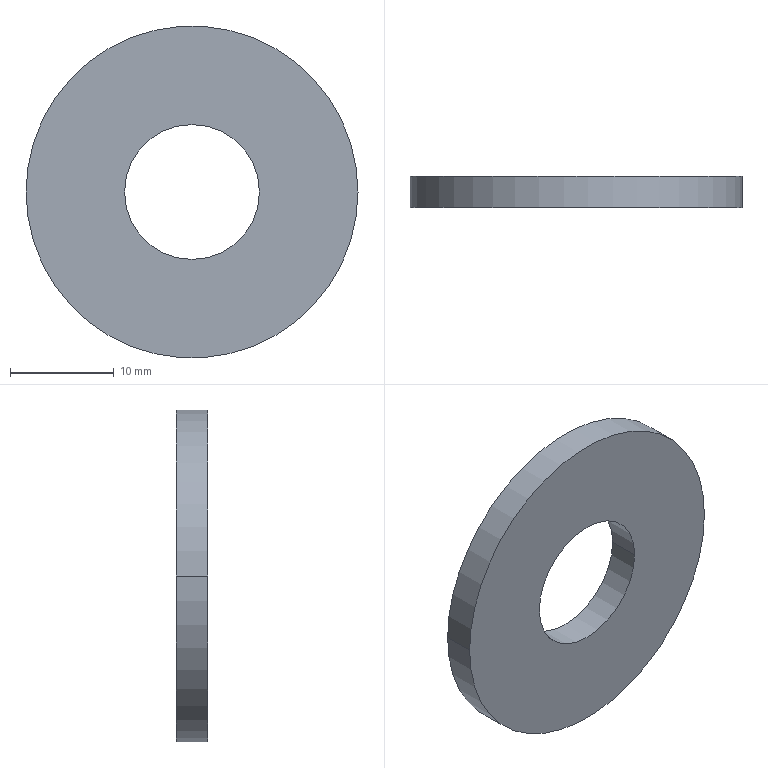Part | STEP file | LIB_26379326_WASHER_M12 | 1 solid | 6 faces | box 32 x 3 x 32 mm | volume 2015 mm3 | cylinder 4 | plane 2 | commonest cylinder face diameters 13 x2 32 x2
STEP:
#1=CARTESIAN_POINT('',(0.,0.,0.));
#2=DIRECTION('',(0.,0.,1.));
#3=DIRECTION('',(1.,0.,0.));
#4=AXIS2_PLACEMENT_3D('',#1,#2,#3);
#5=CARTESIAN_POINT('',(16.,0.,0.));
#6=VERTEX_POINT('',#5);
#7=CARTESIAN_POINT('',(-16.,0.,0.));
#8=VERTEX_POINT('',#7);
#9=CARTESIAN_POINT('',(0.,0.,0.));
#10=DIRECTION('',(0.,1.,0.));
#11=DIRECTION('',(1.,0.,0.));
#12=AXIS2_PLACEMENT_3D('',#9,#10,#11);
#13=CIRCLE('',#12,16.);
#14=CARTESIAN_POINT('',(0.,0.,0.));
#15=DIRECTION('',(0.,1.,0.));
#16=DIRECTION('',(1.,0.,0.));
#17=AXIS2_PLACEMENT_3D('',#14,#15,#16);
#18=PLANE('',#17);
#19=CARTESIAN_POINT('',(0.,0.));
#20=DIRECTION('',(1.,0.));
#21=AXIS2_PLACEMENT_2D('',#19,#20);
#22=CIRCLE('',#21,16.);
#23=(GEOMETRIC_REPRESENTATION_CONTEXT(2)PARAMETRIC_REPRESENTATION_CONTEXT()REPRESENTATION_CONTEXT('',''));
#24=DEFINITIONAL_REPRESENTATION('',(#22),#23);
#25=PCURVE('',#18,#24);
#26=CARTESIAN_POINT('',(0.,0.,0.));
#27=DIRECTION('',(0.,1.,0.));
#28=DIRECTION('',(1.,0.,0.));
#29=AXIS2_PLACEMENT_3D('',#26,#27,#28);
#30=CYLINDRICAL_SURFACE('',#29,16.);
#31=CARTESIAN_POINT('',(0.,0.));
#32=DIRECTION('',(1.,0.));
#33=VECTOR('',#32,1.);
#34=LINE('',#31,#33);
#35=(GEOMETRIC_REPRESENTATION_CONTEXT(2)PARAMETRIC_REPRESENTATION_CONTEXT()REPRESENTATION_CONTEXT('',''));
#36=DEFINITIONAL_REPRESENTATION('',(#34),#35);
#37=PCURVE('',#30,#36);
#38=SURFACE_CURVE('',#13,(#25,#37),.PCURVE_S1.);
#39=EDGE_CURVE('',#6,#8,#38,.T.);
#40=ORIENTED_EDGE('',*,*,#39,.T.);
#41=CARTESIAN_POINT('',(0.,0.,0.));
#42=DIRECTION('',(0.,1.,0.));
#43=DIRECTION('',(-1.,0.,0.));
#44=AXIS2_PLACEMENT_3D('',#41,#42,#43);
#45=CIRCLE('',#44,16.);
#46=CARTESIAN_POINT('',(0.,0.));
#47=DIRECTION('',(-1.,0.));
#48=AXIS2_PLACEMENT_2D('',#46,#47);
#49=CIRCLE('',#48,16.);
#50=(GEOMETRIC_REPRESENTATION_CONTEXT(2)PARAMETRIC_REPRESENTATION_CONTEXT()REPRESENTATION_CONTEXT('',''));
#51=DEFINITIONAL_REPRESENTATION('',(#49),#50);
#52=PCURVE('',#18,#51);
#53=CARTESIAN_POINT('',(0.,0.,0.));
#54=DIRECTION('',(0.,1.,0.));
#55=DIRECTION('',(1.,0.,0.));
#56=AXIS2_PLACEMENT_3D('',#53,#54,#55);
#57=CYLINDRICAL_SURFACE('',#56,16.);
#58=CARTESIAN_POINT('',(3.142,0.));
#59=DIRECTION('',(1.,0.));
#60=VECTOR('',#59,1.);
#61=LINE('',#58,#60);
#62=(GEOMETRIC_REPRESENTATION_CONTEXT(2)PARAMETRIC_REPRESENTATION_CONTEXT()REPRESENTATION_CONTEXT('',''));
#63=DEFINITIONAL_REPRESENTATION('',(#61),#62);
#64=PCURVE('',#57,#63);
#65=SURFACE_CURVE('',#45,(#52,#64),.PCURVE_S1.);
#66=EDGE_CURVE('',#8,#6,#65,.T.);
#67=ORIENTED_EDGE('',*,*,#66,.T.);
#68=EDGE_LOOP('',(#40,#67));
#69=FACE_BOUND('',#68,.F.);
#70=CARTESIAN_POINT('',(6.5,0.,0.));
#71=VERTEX_POINT('',#70);
#72=CARTESIAN_POINT('',(-6.5,0.,0.));
#73=VERTEX_POINT('',#72);
#74=CARTESIAN_POINT('',(0.,0.,0.));
#75=DIRECTION('',(0.,-1.,0.));
#76=DIRECTION('',(1.,0.,0.));
#77=AXIS2_PLACEMENT_3D('',#74,#75,#76);
#78=CIRCLE('',#77,6.5);
#79=CARTESIAN_POINT('',(6.5,0.));
#80=CARTESIAN_POINT('',(6.5,-11.258));
#81=CARTESIAN_POINT('',(-3.25,-5.629));
#82=CARTESIAN_POINT('',(-13.,0.));
#83=CARTESIAN_POINT('',(-3.25,5.629));
#84=CARTESIAN_POINT('',(6.5,11.258));
#85=CARTESIAN_POINT('',(6.5,0.));
#86=(BOUNDED_CURVE()B_SPLINE_CURVE(2,(#79,#80,#81,#82,#83,#84,#85),.UNSPECIFIED.,.T.,.F.)B_SPLINE_CURVE_WITH_KNOTS((1,2,2,2,2,1),(-2.094,0.,2.094,4.189,6.283,8.378),.UNSPECIFIED.)CURVE()GEOMETRIC_REPRESENTATION_ITEM()RATIONAL_B_SPLINE_CURVE((1.,0.5,1.,0.5,1.,0.5,1.))REPRESENTATION_ITEM(''));
#87=(GEOMETRIC_REPRESENTATION_CONTEXT(2)PARAMETRIC_REPRESENTATION_CONTEXT()REPRESENTATION_CONTEXT('',''));
#88=DEFINITIONAL_REPRESENTATION('',(#86),#87);
#89=PCURVE('',#18,#88);
#90=CARTESIAN_POINT('',(0.,0.,0.));
#91=DIRECTION('',(0.,1.,0.));
#92=DIRECTION('',(1.,0.,0.));
#93=AXIS2_PLACEMENT_3D('',#90,#91,#92);
#94=CYLINDRICAL_SURFACE('',#93,6.5);
#95=CARTESIAN_POINT('',(6.283,0.));
#96=DIRECTION('',(-1.,0.));
#97=VECTOR('',#96,1.);
#98=LINE('',#95,#97);
#99=(GEOMETRIC_REPRESENTATION_CONTEXT(2)PARAMETRIC_REPRESENTATION_CONTEXT()REPRESENTATION_CONTEXT('',''));
#100=DEFINITIONAL_REPRESENTATION('',(#98),#99);
#101=PCURVE('',#94,#100);
#102=SURFACE_CURVE('',#78,(#89,#101),.PCURVE_S1.);
#103=EDGE_CURVE('',#71,#73,#102,.T.);
#104=ORIENTED_EDGE('',*,*,#103,.T.);
#105=CARTESIAN_POINT('',(0.,0.,0.));
#106=DIRECTION('',(0.,-1.,0.));
#107=DIRECTION('',(-1.,0.,0.));
#108=AXIS2_PLACEMENT_3D('',#105,#106,#107);
#109=CIRCLE('',#108,6.5);
#110=CARTESIAN_POINT('',(-6.5,0.));
#111=CARTESIAN_POINT('',(-6.5,11.258));
#112=CARTESIAN_POINT('',(3.25,5.629));
#113=CARTESIAN_POINT('',(13.,0.));
#114=CARTESIAN_POINT('',(3.25,-5.629));
#115=CARTESIAN_POINT('',(-6.5,-11.258));
#116=CARTESIAN_POINT('',(-6.5,0.));
#117=(BOUNDED_CURVE()B_SPLINE_CURVE(2,(#110,#111,#112,#113,#114,#115,#116),.UNSPECIFIED.,.T.,.F.)B_SPLINE_CURVE_WITH_KNOTS((1,2,2,2,2,1),(-2.094,0.,2.094,4.189,6.283,8.378),.UNSPECIFIED.)CURVE()GEOMETRIC_REPRESENTATION_ITEM()RATIONAL_B_SPLINE_CURVE((1.,0.5,1.,0.5,1.,0.5,1.))REPRESENTATION_ITEM(''));
#118=(GEOMETRIC_REPRESENTATION_CONTEXT(2)PARAMETRIC_REPRESENTATION_CONTEXT()REPRESENTATION_CONTEXT('',''));
#119=DEFINITIONAL_REPRESENTATION('',(#117),#118);
#120=PCURVE('',#18,#119);
#121=CARTESIAN_POINT('',(0.,0.,0.));
#122=DIRECTION('',(0.,1.,0.));
#123=DIRECTION('',(1.,0.,0.));
#124=AXIS2_PLACEMENT_3D('',#121,#122,#123);
#125=CYLINDRICAL_SURFACE('',#124,6.5);
#126=CARTESIAN_POINT('',(3.142,0.));
#127=DIRECTION('',(-1.,0.));
#128=VECTOR('',#127,1.);
#129=LINE('',#126,#128);
#130=(GEOMETRIC_REPRESENTATION_CONTEXT(2)PARAMETRIC_REPRESENTATION_CONTEXT()REPRESENTATION_CONTEXT('',''));
#131=DEFINITIONAL_REPRESENTATION('',(#129),#130);
#132=PCURVE('',#125,#131);
#133=SURFACE_CURVE('',#109,(#120,#132),.PCURVE_S1.);
#134=EDGE_CURVE('',#73,#71,#133,.T.);
#135=ORIENTED_EDGE('',*,*,#134,.T.);
#136=EDGE_LOOP('',(#104,#135));
#137=FACE_BOUND('',#136,.F.);
#138=ADVANCED_FACE('',(#69,#137),#18,.F.);
#139=CARTESIAN_POINT('',(-16.,3.,0.));
#140=VERTEX_POINT('',#139);
#141=CARTESIAN_POINT('',(-16.,0.,0.));
#142=DIRECTION('',(0.,1.,0.));
#143=VECTOR('',#142,1.);
#144=LINE('',#141,#143);
#145=CARTESIAN_POINT('',(3.142,0.));
#146=DIRECTION('',(0.,1.));
#147=VECTOR('',#146,1.);
#148=LINE('',#145,#147);
#149=(GEOMETRIC_REPRESENTATION_CONTEXT(2)PARAMETRIC_REPRESENTATION_CONTEXT()REPRESENTATION_CONTEXT('',''));
#150=DEFINITIONAL_REPRESENTATION('',(#148),#149);
#151=PCURVE('',#30,#150);
#152=CARTESIAN_POINT('',(3.142,0.));
#153=DIRECTION('',(0.,1.));
#154=VECTOR('',#153,1.);
#155=LINE('',#152,#154);
#156=(GEOMETRIC_REPRESENTATION_CONTEXT(2)PARAMETRIC_REPRESENTATION_CONTEXT()REPRESENTATION_CONTEXT('',''));
#157=DEFINITIONAL_REPRESENTATION('',(#155),#156);
#158=PCURVE('',#57,#157);
#159=SURFACE_CURVE('',#144,(#151,#158),.PCURVE_S1.);
#160=EDGE_CURVE('',#8,#140,#159,.T.);
#161=ORIENTED_EDGE('',*,*,#160,.T.);
#162=CARTESIAN_POINT('',(16.,3.,0.));
#163=VERTEX_POINT('',#162);
#164=CARTESIAN_POINT('',(0.,3.,0.));
#165=DIRECTION('',(0.,1.,0.));
#166=DIRECTION('',(1.,0.,0.));
#167=AXIS2_PLACEMENT_3D('',#164,#165,#166);
#168=CIRCLE('',#167,16.);
#169=CARTESIAN_POINT('',(0.,3.));
#170=DIRECTION('',(1.,0.));
#171=VECTOR('',#170,1.);
#172=LINE('',#169,#171);
#173=(GEOMETRIC_REPRESENTATION_CONTEXT(2)PARAMETRIC_REPRESENTATION_CONTEXT()REPRESENTATION_CONTEXT('',''));
#174=DEFINITIONAL_REPRESENTATION('',(#172),#173);
#175=PCURVE('',#30,#174);
#176=CARTESIAN_POINT('',(0.,3.,0.));
#177=DIRECTION('',(0.,1.,0.));
#178=DIRECTION('',(1.,0.,0.));
#179=AXIS2_PLACEMENT_3D('',#176,#177,#178);
#180=PLANE('',#179);
#181=CARTESIAN_POINT('',(0.,0.));
#182=DIRECTION('',(1.,0.));
#183=AXIS2_PLACEMENT_2D('',#181,#182);
#184=CIRCLE('',#183,16.);
#185=(GEOMETRIC_REPRESENTATION_CONTEXT(2)PARAMETRIC_REPRESENTATION_CONTEXT()REPRESENTATION_CONTEXT('',''));
#186=DEFINITIONAL_REPRESENTATION('',(#184),#185);
#187=PCURVE('',#180,#186);
#188=SURFACE_CURVE('',#168,(#175,#187),.PCURVE_S1.);
#189=EDGE_CURVE('',#163,#140,#188,.T.);
#190=ORIENTED_EDGE('',*,*,#189,.F.);
#191=CARTESIAN_POINT('',(16.,0.,0.));
#192=DIRECTION('',(0.,1.,0.));
#193=VECTOR('',#192,1.);
#194=LINE('',#191,#193);
#195=CARTESIAN_POINT('',(0.,0.));
#196=DIRECTION('',(0.,1.));
#197=VECTOR('',#196,1.);
#198=LINE('',#195,#197);
#199=(GEOMETRIC_REPRESENTATION_CONTEXT(2)PARAMETRIC_REPRESENTATION_CONTEXT()REPRESENTATION_CONTEXT('',''));
#200=DEFINITIONAL_REPRESENTATION('',(#198),#199);
#201=PCURVE('',#30,#200);
#202=CARTESIAN_POINT('',(6.283,0.));
#203=DIRECTION('',(0.,1.));
#204=VECTOR('',#203,1.);
#205=LINE('',#202,#204);
#206=(GEOMETRIC_REPRESENTATION_CONTEXT(2)PARAMETRIC_REPRESENTATION_CONTEXT()REPRESENTATION_CONTEXT('',''));
#207=DEFINITIONAL_REPRESENTATION('',(#205),#206);
#208=PCURVE('',#57,#207);
#209=SURFACE_CURVE('',#194,(#201,#208),.PCURVE_S1.);
#210=EDGE_CURVE('',#6,#163,#209,.T.);
#211=ORIENTED_EDGE('',*,*,#210,.F.);
#212=ORIENTED_EDGE('',*,*,#39,.T.);
#213=EDGE_LOOP('',(#161,#190,#211,#212));
#214=FACE_BOUND('',#213,.T.);
#215=ADVANCED_FACE('',(#214),#30,.T.);
#216=ORIENTED_EDGE('',*,*,#210,.T.);
#217=CARTESIAN_POINT('',(0.,3.,0.));
#218=DIRECTION('',(0.,1.,0.));
#219=DIRECTION('',(-1.,0.,0.));
#220=AXIS2_PLACEMENT_3D('',#217,#218,#219);
#221=CIRCLE('',#220,16.);
#222=CARTESIAN_POINT('',(3.142,3.));
#223=DIRECTION('',(1.,0.));
#224=VECTOR('',#223,1.);
#225=LINE('',#222,#224);
#226=(GEOMETRIC_REPRESENTATION_CONTEXT(2)PARAMETRIC_REPRESENTATION_CONTEXT()REPRESENTATION_CONTEXT('',''));
#227=DEFINITIONAL_REPRESENTATION('',(#225),#226);
#228=PCURVE('',#57,#227);
#229=CARTESIAN_POINT('',(0.,0.));
#230=DIRECTION('',(-1.,0.));
#231=AXIS2_PLACEMENT_2D('',#229,#230);
#232=CIRCLE('',#231,16.);
#233=(GEOMETRIC_REPRESENTATION_CONTEXT(2)PARAMETRIC_REPRESENTATION_CONTEXT()REPRESENTATION_CONTEXT('',''));
#234=DEFINITIONAL_REPRESENTATION('',(#232),#233);
#235=PCURVE('',#180,#234);
#236=SURFACE_CURVE('',#221,(#228,#235),.PCURVE_S1.);
#237=EDGE_CURVE('',#140,#163,#236,.T.);
#238=ORIENTED_EDGE('',*,*,#237,.F.);
#239=ORIENTED_EDGE('',*,*,#160,.F.);
#240=ORIENTED_EDGE('',*,*,#66,.T.);
#241=EDGE_LOOP('',(#216,#238,#239,#240));
#242=FACE_BOUND('',#241,.T.);
#243=ADVANCED_FACE('',(#242),#57,.T.);
#244=ORIENTED_EDGE('',*,*,#189,.F.);
#245=ORIENTED_EDGE('',*,*,#237,.F.);
#246=EDGE_LOOP('',(#244,#245));
#247=FACE_BOUND('',#246,.F.);
#248=CARTESIAN_POINT('',(6.5,3.,0.));
#249=VERTEX_POINT('',#248);
#250=CARTESIAN_POINT('',(-6.5,3.,0.));
#251=VERTEX_POINT('',#250);
#252=CARTESIAN_POINT('',(0.,3.,0.));
#253=DIRECTION('',(0.,-1.,0.));
#254=DIRECTION('',(1.,0.,0.));
#255=AXIS2_PLACEMENT_3D('',#252,#253,#254);
#256=CIRCLE('',#255,6.5);
#257=CARTESIAN_POINT('',(6.5,0.));
#258=CARTESIAN_POINT('',(6.5,-11.258));
#259=CARTESIAN_POINT('',(-3.25,-5.629));
#260=CARTESIAN_POINT('',(-13.,0.));
#261=CARTESIAN_POINT('',(-3.25,5.629));
#262=CARTESIAN_POINT('',(6.5,11.258));
#263=CARTESIAN_POINT('',(6.5,0.));
#264=(BOUNDED_CURVE()B_SPLINE_CURVE(2,(#257,#258,#259,#260,#261,#262,#263),.UNSPECIFIED.,.T.,.F.)B_SPLINE_CURVE_WITH_KNOTS((1,2,2,2,2,1),(-2.094,0.,2.094,4.189,6.283,8.378),.UNSPECIFIED.)CURVE()GEOMETRIC_REPRESENTATION_ITEM()RATIONAL_B_SPLINE_CURVE((1.,0.5,1.,0.5,1.,0.5,1.))REPRESENTATION_ITEM(''));
#265=(GEOMETRIC_REPRESENTATION_CONTEXT(2)PARAMETRIC_REPRESENTATION_CONTEXT()REPRESENTATION_CONTEXT('',''));
#266=DEFINITIONAL_REPRESENTATION('',(#264),#265);
#267=PCURVE('',#180,#266);
#268=CARTESIAN_POINT('',(6.283,3.));
#269=DIRECTION('',(-1.,0.));
#270=VECTOR('',#269,1.);
#271=LINE('',#268,#270);
#272=(GEOMETRIC_REPRESENTATION_CONTEXT(2)PARAMETRIC_REPRESENTATION_CONTEXT()REPRESENTATION_CONTEXT('',''));
#273=DEFINITIONAL_REPRESENTATION('',(#271),#272);
#274=PCURVE('',#94,#273);
#275=SURFACE_CURVE('',#256,(#267,#274),.PCURVE_S1.);
#276=EDGE_CURVE('',#249,#251,#275,.T.);
#277=ORIENTED_EDGE('',*,*,#276,.F.);
#278=CARTESIAN_POINT('',(0.,3.,0.));
#279=DIRECTION('',(0.,-1.,0.));
#280=DIRECTION('',(-1.,0.,0.));
#281=AXIS2_PLACEMENT_3D('',#278,#279,#280);
#282=CIRCLE('',#281,6.5);
#283=CARTESIAN_POINT('',(-6.5,0.));
#284=CARTESIAN_POINT('',(-6.5,11.258));
#285=CARTESIAN_POINT('',(3.25,5.629));
#286=CARTESIAN_POINT('',(13.,0.));
#287=CARTESIAN_POINT('',(3.25,-5.629));
#288=CARTESIAN_POINT('',(-6.5,-11.258));
#289=CARTESIAN_POINT('',(-6.5,0.));
#290=(BOUNDED_CURVE()B_SPLINE_CURVE(2,(#283,#284,#285,#286,#287,#288,#289),.UNSPECIFIED.,.T.,.F.)B_SPLINE_CURVE_WITH_KNOTS((1,2,2,2,2,1),(-2.094,0.,2.094,4.189,6.283,8.378),.UNSPECIFIED.)CURVE()GEOMETRIC_REPRESENTATION_ITEM()RATIONAL_B_SPLINE_CURVE((1.,0.5,1.,0.5,1.,0.5,1.))REPRESENTATION_ITEM(''));
#291=(GEOMETRIC_REPRESENTATION_CONTEXT(2)PARAMETRIC_REPRESENTATION_CONTEXT()REPRESENTATION_CONTEXT('',''));
#292=DEFINITIONAL_REPRESENTATION('',(#290),#291);
#293=PCURVE('',#180,#292);
#294=CARTESIAN_POINT('',(3.142,3.));
#295=DIRECTION('',(-1.,0.));
#296=VECTOR('',#295,1.);
#297=LINE('',#294,#296);
#298=(GEOMETRIC_REPRESENTATION_CONTEXT(2)PARAMETRIC_REPRESENTATION_CONTEXT()REPRESENTATION_CONTEXT('',''));
#299=DEFINITIONAL_REPRESENTATION('',(#297),#298);
#300=PCURVE('',#125,#299);
#301=SURFACE_CURVE('',#282,(#293,#300),.PCURVE_S1.);
#302=EDGE_CURVE('',#251,#249,#301,.T.);
#303=ORIENTED_EDGE('',*,*,#302,.F.);
#304=EDGE_LOOP('',(#277,#303));
#305=FACE_BOUND('',#304,.F.);
#306=ADVANCED_FACE('',(#247,#305),#180,.T.);
#307=ORIENTED_EDGE('',*,*,#103,.F.);
#308=CARTESIAN_POINT('',(6.5,0.,0.));
#309=DIRECTION('',(0.,1.,0.));
#310=VECTOR('',#309,1.);
#311=LINE('',#308,#310);
#312=CARTESIAN_POINT('',(6.283,0.));
#313=DIRECTION('',(0.,1.));
#314=VECTOR('',#313,1.);
#315=LINE('',#312,#314);
#316=(GEOMETRIC_REPRESENTATION_CONTEXT(2)PARAMETRIC_REPRESENTATION_CONTEXT()REPRESENTATION_CONTEXT('',''));
#317=DEFINITIONAL_REPRESENTATION('',(#315),#316);
#318=PCURVE('',#94,#317);
#319=CARTESIAN_POINT('',(0.,0.));
#320=DIRECTION('',(0.,1.));
#321=VECTOR('',#320,1.);
#322=LINE('',#319,#321);
#323=(GEOMETRIC_REPRESENTATION_CONTEXT(2)PARAMETRIC_REPRESENTATION_CONTEXT()REPRESENTATION_CONTEXT('',''));
#324=DEFINITIONAL_REPRESENTATION('',(#322),#323);
#325=PCURVE('',#125,#324);
#326=SURFACE_CURVE('',#311,(#318,#325),.PCURVE_S1.);
#327=EDGE_CURVE('',#71,#249,#326,.T.);
#328=ORIENTED_EDGE('',*,*,#327,.T.);
#329=ORIENTED_EDGE('',*,*,#276,.T.);
#330=CARTESIAN_POINT('',(-6.5,0.,0.));
#331=DIRECTION('',(0.,1.,0.));
#332=VECTOR('',#331,1.);
#333=LINE('',#330,#332);
#334=CARTESIAN_POINT('',(3.142,0.));
#335=DIRECTION('',(0.,1.));
#336=VECTOR('',#335,1.);
#337=LINE('',#334,#336);
#338=(GEOMETRIC_REPRESENTATION_CONTEXT(2)PARAMETRIC_REPRESENTATION_CONTEXT()REPRESENTATION_CONTEXT('',''));
#339=DEFINITIONAL_REPRESENTATION('',(#337),#338);
#340=PCURVE('',#94,#339);
#341=CARTESIAN_POINT('',(3.142,0.));
#342=DIRECTION('',(0.,1.));
#343=VECTOR('',#342,1.);
#344=LINE('',#341,#343);
#345=(GEOMETRIC_REPRESENTATION_CONTEXT(2)PARAMETRIC_REPRESENTATION_CONTEXT()REPRESENTATION_CONTEXT('',''));
#346=DEFINITIONAL_REPRESENTATION('',(#344),#345);
#347=PCURVE('',#125,#346);
#348=SURFACE_CURVE('',#333,(#340,#347),.PCURVE_S1.);
#349=EDGE_CURVE('',#73,#251,#348,.T.);
#350=ORIENTED_EDGE('',*,*,#349,.F.);
#351=EDGE_LOOP('',(#307,#328,#329,#350));
#352=FACE_BOUND('',#351,.F.);
#353=ADVANCED_FACE('',(#352),#94,.F.);
#354=ORIENTED_EDGE('',*,*,#134,.F.);
#355=ORIENTED_EDGE('',*,*,#349,.T.);
#356=ORIENTED_EDGE('',*,*,#302,.T.);
#357=ORIENTED_EDGE('',*,*,#327,.F.);
#358=EDGE_LOOP('',(#354,#355,#356,#357));
#359=FACE_BOUND('',#358,.F.);
#360=ADVANCED_FACE('',(#359),#125,.F.);
#361=CLOSED_SHELL('',(#138,#215,#243,#306,#353,#360));
#362=MANIFOLD_SOLID_BREP('',#361);
#363=(LENGTH_UNIT()NAMED_UNIT(*)SI_UNIT(.MILLI.,.METRE.));
#364=UNCERTAINTY_MEASURE_WITH_UNIT(LENGTH_MEASURE(0.0000001),#363,'','');
#365=(NAMED_UNIT(*)PLANE_ANGLE_UNIT()SI_UNIT($,.RADIAN.));
#366=(NAMED_UNIT(*)SI_UNIT($,.STERADIAN.)SOLID_ANGLE_UNIT());
#367=(GEOMETRIC_REPRESENTATION_CONTEXT(3)GLOBAL_UNCERTAINTY_ASSIGNED_CONTEXT((#364))GLOBAL_UNIT_ASSIGNED_CONTEXT((#363,#365,#366))REPRESENTATION_CONTEXT('',''));
#368=ADVANCED_BREP_SHAPE_REPRESENTATION('',(#4,#362),#367);